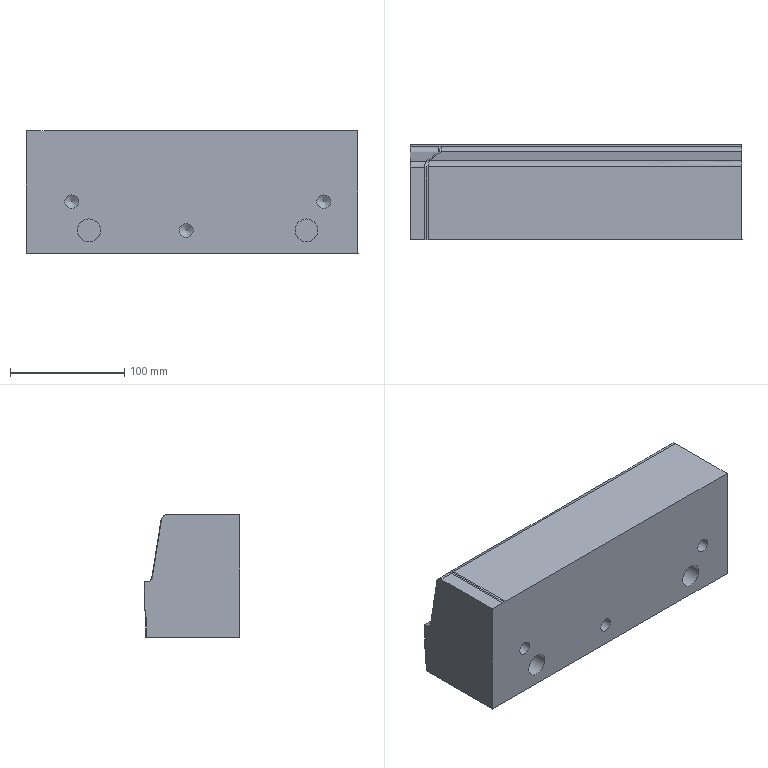Part | NX | features solid 2 | 1 solid | 33 faces | box 290 x 83.721 x 107.133 mm | volume 2375336 mm3 | plane 12 | cylinder 10 | spline 8 | cone 3 | commonest cylinder face diameters 12 x5 10 x3 20 x2
STEP:
#1=CARTESIAN_POINT('',(-215.,-160.,-50.));
#2=VERTEX_POINT('',#1);
#3=CARTESIAN_POINT('',(75.,-160.,-50.));
#4=VERTEX_POINT('',#3);
#5=CARTESIAN_POINT('',(-571.479,-160.,-50.));
#6=DIRECTION('',(1.,0.,0.));
#7=VECTOR('',#6,1000.);
#8=LINE('',#5,#7);
#9=EDGE_CURVE('',#2,#4,#8,.T.);
#10=ORIENTED_EDGE('',*,*,#9,.F.);
#11=CARTESIAN_POINT('',(-215.,-78.115,-50.));
#12=VERTEX_POINT('',#11);
#13=CARTESIAN_POINT('',(-215.,-75.471,-50.));
#14=DIRECTION('',(0.,1.,0.));
#15=VECTOR('',#14,1000.);
#16=LINE('',#13,#15);
#17=EDGE_CURVE('',#2,#12,#16,.T.);
#18=ORIENTED_EDGE('',*,*,#17,.T.);
#19=CARTESIAN_POINT('',(75.,-77.708,-50.));
#20=VERTEX_POINT('',#19);
#21=CARTESIAN_POINT('',(-215.,-78.115,-50.));
#22=CARTESIAN_POINT('',(-211.979,-78.116,-50.));
#23=CARTESIAN_POINT('',(-207.448,-78.118,-50.));
#24=CARTESIAN_POINT('',(-201.406,-78.119,-50.));
#25=CARTESIAN_POINT('',(-197.63,-78.126,-50.));
#26=CARTESIAN_POINT('',(-194.609,-78.116,-50.));
#27=CARTESIAN_POINT('',(-192.344,-78.15,-50.));
#28=CARTESIAN_POINT('',(-190.078,-78.04,-50.));
#29=CARTESIAN_POINT('',(-187.813,-77.65,-50.));
#30=CARTESIAN_POINT('',(-185.547,-77.717,-50.));
#31=CARTESIAN_POINT('',(-182.527,-77.699,-50.));
#32=CARTESIAN_POINT('',(-177.24,-77.699,-50.));
#33=CARTESIAN_POINT('',(-169.688,-77.703,-50.));
#34=CARTESIAN_POINT('',(-157.605,-77.713,-50.));
#35=CARTESIAN_POINT('',(-136.459,-77.708,-50.));
#36=CARTESIAN_POINT('',(-106.25,-77.699,-50.));
#37=CARTESIAN_POINT('',(-57.917,-77.699,-50.));
#38=CARTESIAN_POINT('',(2.5,-77.706,-50.));
#39=CARTESIAN_POINT('',(50.833,-77.708,-50.));
#40=CARTESIAN_POINT('',(75.,-77.708,-50.));
#41=B_SPLINE_CURVE_WITH_KNOTS('',3,(#21,#22,#23,#24,#25,#26,#27,#28,#29,#30,#31,#32,#33,#34,#35,#36,#37,#38,#39,#40),.UNSPECIFIED.,.F.,.F.,(4,1,1,1,1,1,1,1,1,1,1,1,1,1,1,1,1,4),(0.1494,0.1584,0.163,0.1675,0.1698,0.172,0.1743,0.1766,0.1788,0.1811,0.1856,0.1947,0.2037,0.2219,0.2581,0.2944,0.3669,0.4394),.UNSPECIFIED.);
#42=EDGE_CURVE('',#12,#20,#41,.T.);
#43=ORIENTED_EDGE('',*,*,#42,.T.);
#44=CARTESIAN_POINT('',(75.,-160.,-50.));
#45=DIRECTION('',(0.,1.,0.));
#46=VECTOR('',#45,1000.);
#47=LINE('',#44,#46);
#48=EDGE_CURVE('',#4,#20,#47,.T.);
#49=ORIENTED_EDGE('',*,*,#48,.F.);
#50=EDGE_LOOP('',(#10,#18,#43,#49));
#51=FACE_BOUND('',#50,.T.);
#52=CARTESIAN_POINT('',(-571.479,-75.471,-50.));
#53=DIRECTION('',(0.,0.,-1.));
#54=DIRECTION('',(-1.,0.,0.));
#55=AXIS2_PLACEMENT_3D('',#52,#53,#54);
#56=PLANE('',#55);
#57=ADVANCED_FACE('',(#51),#56,.T.);
#58=ORIENTED_EDGE('',*,*,#42,.F.);
#59=CARTESIAN_POINT('',(-215.,-77.915,-26.496));
#60=VERTEX_POINT('',#59);
#61=CARTESIAN_POINT('',(-215.,-78.015,-38.265));
#62=DIRECTION('',(0.,-0.008536,-1.));
#63=VECTOR('',#62,1000.);
#64=LINE('',#61,#63);
#65=EDGE_CURVE('',#12,#60,#64,.F.);
#66=ORIENTED_EDGE('',*,*,#65,.T.);
#67=CARTESIAN_POINT('',(75.,-77.507,-26.5));
#68=VERTEX_POINT('',#67);
#69=CARTESIAN_POINT('',(-215.,-77.915,-26.496));
#70=CARTESIAN_POINT('',(-211.979,-77.915,-26.496));
#71=CARTESIAN_POINT('',(-207.448,-77.918,-26.496));
#72=CARTESIAN_POINT('',(-201.406,-77.918,-26.496));
#73=CARTESIAN_POINT('',(-197.63,-77.925,-26.496));
#74=CARTESIAN_POINT('',(-194.609,-77.916,-26.496));
#75=CARTESIAN_POINT('',(-192.344,-77.949,-26.496));
#76=CARTESIAN_POINT('',(-190.078,-77.839,-26.497));
#77=CARTESIAN_POINT('',(-187.813,-77.449,-26.5));
#78=CARTESIAN_POINT('',(-185.547,-77.516,-26.499));
#79=CARTESIAN_POINT('',(-182.527,-77.499,-26.5));
#80=CARTESIAN_POINT('',(-177.24,-77.499,-26.5));
#81=CARTESIAN_POINT('',(-169.688,-77.502,-26.5));
#82=CARTESIAN_POINT('',(-157.605,-77.512,-26.5));
#83=CARTESIAN_POINT('',(-136.459,-77.507,-26.5));
#84=CARTESIAN_POINT('',(-106.25,-77.499,-26.5));
#85=CARTESIAN_POINT('',(-57.917,-77.498,-26.5));
#86=CARTESIAN_POINT('',(2.5,-77.505,-26.5));
#87=CARTESIAN_POINT('',(50.833,-77.507,-26.5));
#88=CARTESIAN_POINT('',(75.,-77.507,-26.5));
#89=B_SPLINE_CURVE_WITH_KNOTS('',3,(#69,#70,#71,#72,#73,#74,#75,#76,#77,#78,#79,#80,#81,#82,#83,#84,#85,#86,#87,#88),.UNSPECIFIED.,.F.,.F.,(4,1,1,1,1,1,1,1,1,1,1,1,1,1,1,1,1,4),(0.1353,0.1444,0.1489,0.1535,0.1557,0.158,0.1603,0.1625,0.1648,0.1671,0.1716,0.1807,0.1897,0.2078,0.2441,0.2803,0.3528,0.4253),.UNSPECIFIED.);
#90=EDGE_CURVE('',#60,#68,#89,.T.);
#91=ORIENTED_EDGE('',*,*,#90,.T.);
#92=CARTESIAN_POINT('',(75.,-77.608,-38.267));
#93=DIRECTION('',(0.,-0.008536,-1.));
#94=VECTOR('',#93,1000.);
#95=LINE('',#92,#94);
#96=EDGE_CURVE('',#20,#68,#95,.F.);
#97=ORIENTED_EDGE('',*,*,#96,.F.);
#98=EDGE_LOOP('',(#58,#66,#91,#97));
#99=FACE_BOUND('',#98,.T.);
#100=CARTESIAN_POINT('',(-215.,-77.915,-26.496));
#101=CARTESIAN_POINT('',(-215.,-78.117,-50.141));
#102=CARTESIAN_POINT('',(-211.979,-77.915,-26.496));
#103=CARTESIAN_POINT('',(-211.979,-78.117,-50.141));
#104=CARTESIAN_POINT('',(-207.449,-77.918,-26.496));
#105=CARTESIAN_POINT('',(-207.449,-78.12,-50.141));
#106=CARTESIAN_POINT('',(-201.403,-77.918,-26.496));
#107=CARTESIAN_POINT('',(-201.403,-78.12,-50.141));
#108=CARTESIAN_POINT('',(-197.637,-77.926,-26.496));
#109=CARTESIAN_POINT('',(-197.637,-78.128,-50.141));
#110=CARTESIAN_POINT('',(-194.595,-77.914,-26.496));
#111=CARTESIAN_POINT('',(-194.595,-78.116,-50.141));
#112=CARTESIAN_POINT('',(-192.394,-77.956,-26.496));
#113=CARTESIAN_POINT('',(-192.394,-78.158,-50.141));
#114=CARTESIAN_POINT('',(-189.892,-77.814,-26.497));
#115=CARTESIAN_POINT('',(-189.892,-78.016,-50.142));
#116=CARTESIAN_POINT('',(-187.778,-77.451,-26.5));
#117=CARTESIAN_POINT('',(-187.778,-77.653,-50.145));
#118=CARTESIAN_POINT('',(-185.598,-77.515,-26.499));
#119=CARTESIAN_POINT('',(-185.598,-77.717,-50.145));
#120=CARTESIAN_POINT('',(-182.526,-77.499,-26.5));
#121=CARTESIAN_POINT('',(-182.526,-77.701,-50.145));
#122=CARTESIAN_POINT('',(-177.274,-77.498,-26.5));
#123=CARTESIAN_POINT('',(-177.274,-77.7,-50.145));
#124=CARTESIAN_POINT('',(-169.704,-77.502,-26.5));
#125=CARTESIAN_POINT('',(-169.704,-77.704,-50.145));
#126=CARTESIAN_POINT('',(-157.625,-77.512,-26.5));
#127=CARTESIAN_POINT('',(-157.625,-77.714,-50.145));
#128=CARTESIAN_POINT('',(-136.473,-77.507,-26.5));
#129=CARTESIAN_POINT('',(-136.473,-77.709,-50.145));
#130=CARTESIAN_POINT('',(-106.265,-77.499,-26.5));
#131=CARTESIAN_POINT('',(-106.265,-77.701,-50.145));
#132=CARTESIAN_POINT('',(-57.927,-77.498,-26.5));
#133=CARTESIAN_POINT('',(-57.927,-77.7,-50.145));
#134=CARTESIAN_POINT('',(2.494,-77.505,-26.5));
#135=CARTESIAN_POINT('',(2.494,-77.707,-50.145));
#136=CARTESIAN_POINT('',(50.831,-77.507,-26.5));
#137=CARTESIAN_POINT('',(50.831,-77.709,-50.145));
#138=CARTESIAN_POINT('',(75.,-77.507,-26.5));
#139=CARTESIAN_POINT('',(75.,-77.709,-50.145));
#140=B_SPLINE_SURFACE_WITH_KNOTS('',3,1,((#100,#101),(#102,#103),(#104,#105),(#106,#107),(#108,#109),(#110,#111),(#112,#113),(#114,#115),(#116,#117),(#118,#119),(#120,#121),(#122,#123),(#124,#125),(#126,#127),(#128,#129),(#130,#131),(#132,#133),(#134,#135),(#136,#137),(#138,#139)),.SURF_OF_LINEAR_EXTRUSION.,.F.,.F.,.F.,(4,1,1,1,1,1,1,1,1,1,1,1,1,1,1,1,1,4),(2,2),(0.3592,0.3659,0.3692,0.3725,0.3742,0.3758,0.3775,0.3791,0.3808,0.3825,0.3858,0.3924,0.3991,0.4123,0.4389,0.4654,0.5185,0.5716),(0.,1.),.UNSPECIFIED.);
#141=ADVANCED_FACE('',(#99),#140,.T.);
#142=ORIENTED_EDGE('',*,*,#96,.T.);
#143=CARTESIAN_POINT('',(75.,-76.294,-26.51));
#144=VERTEX_POINT('',#143);
#145=CARTESIAN_POINT('',(75.,-76.914,-26.505));
#146=DIRECTION('',(0.,-1.,0.008536));
#147=VECTOR('',#146,1000.);
#148=LINE('',#145,#147);
#149=EDGE_CURVE('',#144,#68,#148,.T.);
#150=ORIENTED_EDGE('',*,*,#149,.F.);
#151=CARTESIAN_POINT('',(75.,-76.294,-1.509));
#152=VERTEX_POINT('',#151);
#153=CARTESIAN_POINT('',(75.,-76.294,-14.008));
#154=DIRECTION('',(0.,0.,-1.));
#155=VECTOR('',#154,1000.);
#156=LINE('',#153,#155);
#157=EDGE_CURVE('',#152,#144,#156,.T.);
#158=ORIENTED_EDGE('',*,*,#157,.F.);
#159=CARTESIAN_POINT('',(75.,-78.294,-1.492));
#160=VERTEX_POINT('',#159);
#161=CARTESIAN_POINT('',(75.,46.797,-2.56));
#162=DIRECTION('',(0.,1.,-0.008536));
#163=VECTOR('',#162,1000.);
#164=LINE('',#161,#163);
#165=EDGE_CURVE('',#160,#152,#164,.T.);
#166=ORIENTED_EDGE('',*,*,#165,.F.);
#167=CARTESIAN_POINT('',(75.,-83.189,2.72));
#168=VERTEX_POINT('',#167);
#169=CARTESIAN_POINT('',(75.,-78.252,3.508));
#170=DIRECTION('',(-1.,0.,0.));
#171=DIRECTION('',(0.,0.,1.));
#172=AXIS2_PLACEMENT_3D('',#169,#170,#171);
#173=CIRCLE('',#172,5.);
#174=EDGE_CURVE('',#168,#160,#173,.F.);
#175=ORIENTED_EDGE('',*,*,#174,.F.);
#176=CARTESIAN_POINT('',(75.,-91.197,52.92));
#177=VERTEX_POINT('',#176);
#178=CARTESIAN_POINT('',(75.,-87.499,29.736));
#179=DIRECTION('',(0.,0.1575,-0.9875));
#180=VECTOR('',#179,1000.);
#181=LINE('',#178,#180);
#182=EDGE_CURVE('',#177,#168,#181,.T.);
#183=ORIENTED_EDGE('',*,*,#182,.F.);
#184=CARTESIAN_POINT('',(75.,-96.134,57.133));
#185=VERTEX_POINT('',#184);
#186=CARTESIAN_POINT('',(75.,-96.134,52.133));
#187=DIRECTION('',(-1.,0.,0.));
#188=DIRECTION('',(0.,0.,1.));
#189=AXIS2_PLACEMENT_3D('',#186,#187,#188);
#190=CIRCLE('',#189,5.);
#191=EDGE_CURVE('',#177,#185,#190,.F.);
#192=ORIENTED_EDGE('',*,*,#191,.T.);
#193=CARTESIAN_POINT('',(75.,-160.,57.133));
#194=VERTEX_POINT('',#193);
#195=CARTESIAN_POINT('',(75.,-91.869,57.133));
#196=DIRECTION('',(0.,-1.,0.));
#197=VECTOR('',#196,1000.);
#198=LINE('',#195,#197);
#199=EDGE_CURVE('',#185,#194,#198,.T.);
#200=ORIENTED_EDGE('',*,*,#199,.T.);
#201=CARTESIAN_POINT('',(75.,-160.,200.));
#202=DIRECTION('',(0.,0.,1.));
#203=VECTOR('',#202,1000.);
#204=LINE('',#201,#203);
#205=EDGE_CURVE('',#4,#194,#204,.T.);
#206=ORIENTED_EDGE('',*,*,#205,.F.);
#207=ORIENTED_EDGE('',*,*,#48,.T.);
#208=EDGE_LOOP('',(#142,#150,#158,#166,#175,#183,#192,#200,#206,#207));
#209=FACE_BOUND('',#208,.T.);
#210=CARTESIAN_POINT('',(75.,360.,0.));
#211=DIRECTION('',(-1.,0.,0.));
#212=DIRECTION('',(0.,0.,1.));
#213=AXIS2_PLACEMENT_3D('',#210,#211,#212);
#214=PLANE('',#213);
#215=ADVANCED_FACE('',(#209),#214,.F.);
#216=CARTESIAN_POINT('',(-215.,-160.,57.07));
#217=VERTEX_POINT('',#216);
#218=CARTESIAN_POINT('',(-215.,-160.,200.));
#219=DIRECTION('',(0.,0.,1.));
#220=VECTOR('',#219,1000.);
#221=LINE('',#218,#220);
#222=EDGE_CURVE('',#2,#217,#221,.T.);
#223=ORIENTED_EDGE('',*,*,#222,.F.);
#224=ORIENTED_EDGE('',*,*,#9,.T.);
#225=ORIENTED_EDGE('',*,*,#205,.T.);
#226=CARTESIAN_POINT('',(-198.963,-160.,57.133));
#227=VERTEX_POINT('',#226);
#228=CARTESIAN_POINT('',(-705.,-160.,57.133));
#229=DIRECTION('',(1.,0.,0.));
#230=VECTOR('',#229,1000.);
#231=LINE('',#228,#230);
#232=EDGE_CURVE('',#227,#194,#231,.T.);
#233=ORIENTED_EDGE('',*,*,#232,.F.);
#234=CARTESIAN_POINT('',(-200.536,-160.,57.112));
#235=VERTEX_POINT('',#234);
#236=CARTESIAN_POINT('',(-703.043,-160.,50.532));
#237=DIRECTION('',(0.9999,0.,0.01309));
#238=VECTOR('',#237,1000.);
#239=LINE('',#236,#238);
#240=EDGE_CURVE('',#235,#227,#239,.T.);
#241=ORIENTED_EDGE('',*,*,#240,.F.);
#242=CARTESIAN_POINT('',(-202.104,-160.,57.07));
#243=VERTEX_POINT('',#242);
#244=CARTESIAN_POINT('',(-200.536,-160.,57.112));
#245=CARTESIAN_POINT('',(-201.059,-160.,57.095));
#246=CARTESIAN_POINT('',(-201.581,-160.,57.081));
#247=CARTESIAN_POINT('',(-202.104,-160.,57.075));
#248=B_SPLINE_CURVE_WITH_KNOTS('',3,(#244,#245,#246,#247),.UNSPECIFIED.,.F.,.F.,(4,4),(0.006154,0.007723),.UNSPECIFIED.);
#249=EDGE_CURVE('',#243,#235,#248,.F.);
#250=ORIENTED_EDGE('',*,*,#249,.F.);
#251=CARTESIAN_POINT('',(-705.,-160.,57.07));
#252=DIRECTION('',(-1.,0.,0.));
#253=VECTOR('',#252,1000.);
#254=LINE('',#251,#253);
#255=EDGE_CURVE('',#243,#217,#254,.T.);
#256=ORIENTED_EDGE('',*,*,#255,.T.);
#257=EDGE_LOOP('',(#223,#224,#225,#233,#241,#250,#256));
#258=FACE_BOUND('',#257,.T.);
#259=CARTESIAN_POINT('',(45.,-160.,1.));
#260=VERTEX_POINT('',#259);
#261=CARTESIAN_POINT('',(45.,-160.,-5.));
#262=DIRECTION('',(0.,1.,0.));
#263=DIRECTION('',(0.,0.,1.));
#264=AXIS2_PLACEMENT_3D('',#261,#262,#263);
#265=CIRCLE('',#264,6.);
#266=EDGE_CURVE('',#260,#260,#265,.T.);
#267=ORIENTED_EDGE('',*,*,#266,.T.);
#268=EDGE_LOOP('',(#267));
#269=FACE_BOUND('',#268,.T.);
#270=CARTESIAN_POINT('',(-75.,-160.,-24.));
#271=VERTEX_POINT('',#270);
#272=CARTESIAN_POINT('',(-75.,-160.,-30.));
#273=DIRECTION('',(0.,1.,0.));
#274=DIRECTION('',(0.,0.,1.));
#275=AXIS2_PLACEMENT_3D('',#272,#273,#274);
#276=CIRCLE('',#275,6.);
#277=EDGE_CURVE('',#271,#271,#276,.T.);
#278=ORIENTED_EDGE('',*,*,#277,.T.);
#279=EDGE_LOOP('',(#278));
#280=FACE_BOUND('',#279,.T.);
#281=CARTESIAN_POINT('',(-175.,-160.,1.));
#282=VERTEX_POINT('',#281);
#283=CARTESIAN_POINT('',(-175.,-160.,-5.));
#284=DIRECTION('',(0.,1.,0.));
#285=DIRECTION('',(0.,0.,1.));
#286=AXIS2_PLACEMENT_3D('',#283,#284,#285);
#287=CIRCLE('',#286,6.);
#288=EDGE_CURVE('',#282,#282,#287,.T.);
#289=ORIENTED_EDGE('',*,*,#288,.T.);
#290=EDGE_LOOP('',(#289));
#291=FACE_BOUND('',#290,.T.);
#292=CARTESIAN_POINT('',(30.,-160.,-20.));
#293=VERTEX_POINT('',#292);
#294=CARTESIAN_POINT('',(30.,-160.,-30.));
#295=DIRECTION('',(0.,1.,0.));
#296=DIRECTION('',(0.,0.,1.));
#297=AXIS2_PLACEMENT_3D('',#294,#295,#296);
#298=CIRCLE('',#297,10.);
#299=EDGE_CURVE('',#293,#293,#298,.T.);
#300=ORIENTED_EDGE('',*,*,#299,.T.);
#301=EDGE_LOOP('',(#300));
#302=FACE_BOUND('',#301,.T.);
#303=CARTESIAN_POINT('',(-160.,-160.,-20.));
#304=VERTEX_POINT('',#303);
#305=CARTESIAN_POINT('',(-160.,-160.,-30.));
#306=DIRECTION('',(0.,1.,0.));
#307=DIRECTION('',(0.,0.,1.));
#308=AXIS2_PLACEMENT_3D('',#305,#306,#307);
#309=CIRCLE('',#308,10.);
#310=EDGE_CURVE('',#304,#304,#309,.T.);
#311=ORIENTED_EDGE('',*,*,#310,.T.);
#312=EDGE_LOOP('',(#311));
#313=FACE_BOUND('',#312,.T.);
#314=CARTESIAN_POINT('',(-705.,-160.,200.));
#315=DIRECTION('',(0.,1.,0.));
#316=DIRECTION('',(0.,0.,1.));
#317=AXIS2_PLACEMENT_3D('',#314,#315,#316);
#318=PLANE('',#317);
#319=ADVANCED_FACE('',(#258,#269,#280,#291,#302,#313),#318,.F.);
#320=CARTESIAN_POINT('',(-215.,-76.704,-26.506));
#321=VERTEX_POINT('',#320);
#322=CARTESIAN_POINT('',(-215.,-76.914,-26.505));
#323=DIRECTION('',(0.,-1.,0.008536));
#324=VECTOR('',#323,1000.);
#325=LINE('',#322,#324);
#326=EDGE_CURVE('',#321,#60,#325,.T.);
#327=ORIENTED_EDGE('',*,*,#326,.T.);
#328=ORIENTED_EDGE('',*,*,#65,.F.);
#329=ORIENTED_EDGE('',*,*,#17,.F.);
#330=ORIENTED_EDGE('',*,*,#222,.T.);
#331=CARTESIAN_POINT('',(-215.,-96.529,57.07));
#332=VERTEX_POINT('',#331);
#333=CARTESIAN_POINT('',(-215.,-392.264,57.07));
#334=DIRECTION('',(0.,1.,0.));
#335=VECTOR('',#334,1000.);
#336=LINE('',#333,#335);
#337=EDGE_CURVE('',#217,#332,#336,.T.);
#338=ORIENTED_EDGE('',*,*,#337,.T.);
#339=CARTESIAN_POINT('',(-215.,-91.592,52.857));
#340=VERTEX_POINT('',#339);
#341=CARTESIAN_POINT('',(-215.,-96.529,52.07));
#342=DIRECTION('',(-1.,0.,0.));
#343=DIRECTION('',(0.,0.,1.));
#344=AXIS2_PLACEMENT_3D('',#341,#342,#343);
#345=CIRCLE('',#344,5.);
#346=EDGE_CURVE('',#340,#332,#345,.F.);
#347=ORIENTED_EDGE('',*,*,#346,.F.);
#348=CARTESIAN_POINT('',(-215.,-83.595,2.724));
#349=VERTEX_POINT('',#348);
#350=CARTESIAN_POINT('',(-215.,-79.399,-23.581));
#351=DIRECTION('',(0.,0.1575,-0.9875));
#352=VECTOR('',#351,1000.);
#353=LINE('',#350,#352);
#354=EDGE_CURVE('',#340,#349,#353,.T.);
#355=ORIENTED_EDGE('',*,*,#354,.T.);
#356=CARTESIAN_POINT('',(-215.,-78.7,-1.488));
#357=VERTEX_POINT('',#356);
#358=CARTESIAN_POINT('',(-215.,-78.657,3.511));
#359=DIRECTION('',(-1.,0.,0.));
#360=DIRECTION('',(0.,0.,1.));
#361=AXIS2_PLACEMENT_3D('',#358,#359,#360);
#362=CIRCLE('',#361,5.);
#363=EDGE_CURVE('',#349,#357,#362,.F.);
#364=ORIENTED_EDGE('',*,*,#363,.T.);
#365=CARTESIAN_POINT('',(-215.,-76.704,-1.506));
#366=VERTEX_POINT('',#365);
#367=CARTESIAN_POINT('',(-215.,46.797,-2.56));
#368=DIRECTION('',(0.,1.,-0.008536));
#369=VECTOR('',#368,1000.);
#370=LINE('',#367,#369);
#371=EDGE_CURVE('',#357,#366,#370,.T.);
#372=ORIENTED_EDGE('',*,*,#371,.T.);
#373=CARTESIAN_POINT('',(-215.,-76.704,-14.008));
#374=DIRECTION('',(0.,0.,-1.));
#375=VECTOR('',#374,1000.);
#376=LINE('',#373,#375);
#377=EDGE_CURVE('',#366,#321,#376,.T.);
#378=ORIENTED_EDGE('',*,*,#377,.T.);
#379=EDGE_LOOP('',(#327,#328,#329,#330,#338,#347,#355,#364,#372,#378));
#380=FACE_BOUND('',#379,.T.);
#381=CARTESIAN_POINT('',(-215.,360.,0.));
#382=DIRECTION('',(-1.,0.,0.));
#383=DIRECTION('',(0.,0.,1.));
#384=AXIS2_PLACEMENT_3D('',#381,#382,#383);
#385=PLANE('',#384);
#386=ADVANCED_FACE('',(#380),#385,.T.);
#387=CARTESIAN_POINT('',(-199.628,-91.395,52.891));
#388=VERTEX_POINT('',#387);
#389=CARTESIAN_POINT('',(-198.056,-91.197,52.92));
#390=VERTEX_POINT('',#389);
#391=CARTESIAN_POINT('',(-199.628,-91.395,52.894));
#392=CARTESIAN_POINT('',(-199.206,-91.287,52.907));
#393=CARTESIAN_POINT('',(-198.679,-91.197,52.92));
#394=CARTESIAN_POINT('',(-198.056,-91.197,52.92));
#395=B_SPLINE_CURVE_WITH_KNOTS('',3,(#391,#392,#393,#394),.UNSPECIFIED.,.F.,.F.,(4,4),(0.6644,1.),.UNSPECIFIED.);
#396=EDGE_CURVE('',#388,#390,#395,.T.);
#397=ORIENTED_EDGE('',*,*,#396,.T.);
#398=CARTESIAN_POINT('',(-196.309,-89.902,44.803));
#399=VERTEX_POINT('',#398);
#400=CARTESIAN_POINT('',(-196.309,-89.902,44.803));
#401=CARTESIAN_POINT('',(-196.892,-90.333,47.509));
#402=CARTESIAN_POINT('',(-197.474,-90.765,50.215));
#403=CARTESIAN_POINT('',(-198.056,-91.197,52.92));
#404=B_SPLINE_CURVE_WITH_KNOTS('',3,(#400,#401,#402,#403),.UNSPECIFIED.,.F.,.F.,(4,4),(0.,1.),.UNSPECIFIED.);
#405=EDGE_CURVE('',#399,#390,#404,.T.);
#406=ORIENTED_EDGE('',*,*,#405,.F.);
#407=CARTESIAN_POINT('',(-194.188,-88.33,34.95));
#408=VERTEX_POINT('',#407);
#409=CARTESIAN_POINT('',(-194.188,-88.33,34.95));
#410=CARTESIAN_POINT('',(-194.895,-88.854,38.234));
#411=CARTESIAN_POINT('',(-195.602,-89.378,41.518));
#412=CARTESIAN_POINT('',(-196.309,-89.902,44.803));
#413=B_SPLINE_CURVE_WITH_KNOTS('',3,(#409,#410,#411,#412),.UNSPECIFIED.,.F.,.F.,(4,4),(0.,1.),.UNSPECIFIED.);
#414=EDGE_CURVE('',#408,#399,#413,.T.);
#415=ORIENTED_EDGE('',*,*,#414,.F.);
#416=CARTESIAN_POINT('',(-187.251,-83.189,2.72));
#417=VERTEX_POINT('',#416);
#418=CARTESIAN_POINT('',(-187.251,-83.189,2.72));
#419=CARTESIAN_POINT('',(-189.564,-84.903,13.463));
#420=CARTESIAN_POINT('',(-191.876,-86.617,24.207));
#421=CARTESIAN_POINT('',(-194.188,-88.33,34.95));
#422=B_SPLINE_CURVE_WITH_KNOTS('',3,(#418,#419,#420,#421),.UNSPECIFIED.,.F.,.F.,(4,4),(0.,1.),.UNSPECIFIED.);
#423=EDGE_CURVE('',#417,#408,#422,.T.);
#424=ORIENTED_EDGE('',*,*,#423,.F.);
#425=CARTESIAN_POINT('',(-188.891,-83.438,3.013));
#426=VERTEX_POINT('',#425);
#427=CARTESIAN_POINT('',(-188.891,-83.438,3.013));
#428=CARTESIAN_POINT('',(-188.315,-83.277,2.9));
#429=CARTESIAN_POINT('',(-187.761,-83.202,2.803));
#430=CARTESIAN_POINT('',(-187.251,-83.189,2.72));
#431=B_SPLINE_CURVE_WITH_KNOTS('',3,(#427,#428,#429,#430),.UNSPECIFIED.,.F.,.F.,(4,4),(0.,1.),.UNSPECIFIED.);
#432=EDGE_CURVE('',#417,#426,#431,.F.);
#433=ORIENTED_EDGE('',*,*,#432,.T.);
#434=CARTESIAN_POINT('',(-195.756,-88.526,34.905));
#435=VERTEX_POINT('',#434);
#436=CARTESIAN_POINT('',(-195.756,-88.526,34.905));
#437=CARTESIAN_POINT('',(-193.468,-86.83,24.274));
#438=CARTESIAN_POINT('',(-191.18,-85.134,13.643));
#439=CARTESIAN_POINT('',(-188.891,-83.438,3.013));
#440=B_SPLINE_CURVE_WITH_KNOTS('',3,(#436,#437,#438,#439),.UNSPECIFIED.,.F.,.F.,(4,4),(0.,1.),.UNSPECIFIED.);
#441=EDGE_CURVE('',#426,#435,#440,.F.);
#442=ORIENTED_EDGE('',*,*,#441,.T.);
#443=CARTESIAN_POINT('',(-197.877,-90.097,44.758));
#444=VERTEX_POINT('',#443);
#445=CARTESIAN_POINT('',(-190.129,-84.356,8.763));
#446=DIRECTION('',(-0.2079,-0.1541,0.9659));
#447=VECTOR('',#446,1000.);
#448=LINE('',#445,#447);
#449=EDGE_CURVE('',#435,#444,#448,.T.);
#450=ORIENTED_EDGE('',*,*,#449,.T.);
#451=CARTESIAN_POINT('',(-199.628,-91.395,52.894));
#452=CARTESIAN_POINT('',(-199.044,-90.962,50.182));
#453=CARTESIAN_POINT('',(-198.461,-90.53,47.47));
#454=CARTESIAN_POINT('',(-197.877,-90.097,44.758));
#455=B_SPLINE_CURVE_WITH_KNOTS('',3,(#451,#452,#453,#454),.UNSPECIFIED.,.F.,.F.,(4,4),(0.,1.),.UNSPECIFIED.);
#456=EDGE_CURVE('',#444,#388,#455,.F.);
#457=ORIENTED_EDGE('',*,*,#456,.T.);
#458=EDGE_LOOP('',(#397,#406,#415,#424,#433,#442,#450,#457));
#459=FACE_BOUND('',#458,.T.);
#460=CARTESIAN_POINT('',(-188.626,-90.134,8.164));
#461=DIRECTION('',(-0.2079,-0.1541,0.9659));
#462=DIRECTION('',(0.9781,-0.03275,0.2053));
#463=AXIS2_PLACEMENT_3D('',#460,#461,#462);
#464=CYLINDRICAL_SURFACE('',#463,6.);
#465=ADVANCED_FACE('',(#459),#464,.T.);
#466=ORIENTED_EDGE('',*,*,#191,.F.);
#467=CARTESIAN_POINT('',(-198.056,-91.197,52.92));
#468=CARTESIAN_POINT('',(-107.038,-91.197,52.92));
#469=CARTESIAN_POINT('',(-16.019,-91.197,52.92));
#470=CARTESIAN_POINT('',(75.,-91.197,52.92));
#471=B_SPLINE_CURVE_WITH_KNOTS('',3,(#467,#468,#469,#470),.UNSPECIFIED.,.F.,.F.,(4,4),(0.,0.2731),.UNSPECIFIED.);
#472=EDGE_CURVE('',#390,#177,#471,.T.);
#473=ORIENTED_EDGE('',*,*,#472,.F.);
#474=CARTESIAN_POINT('',(-198.963,-96.134,57.132));
#475=VERTEX_POINT('',#474);
#476=CARTESIAN_POINT('',(-198.963,-96.133,57.132));
#477=CARTESIAN_POINT('',(-198.958,-94.944,57.111));
#478=CARTESIAN_POINT('',(-198.774,-92.575,56.253));
#479=CARTESIAN_POINT('',(-198.303,-91.389,54.067));
#480=CARTESIAN_POINT('',(-198.056,-91.197,52.92));
#481=B_SPLINE_CURVE_WITH_KNOTS('',3,(#476,#477,#478,#479,#480),.UNSPECIFIED.,.F.,.F.,(4,1,4),(0.,0.5,1.),.UNSPECIFIED.);
#482=EDGE_CURVE('',#475,#390,#481,.T.);
#483=ORIENTED_EDGE('',*,*,#482,.F.);
#484=CARTESIAN_POINT('',(75.,-96.134,57.133));
#485=CARTESIAN_POINT('',(-16.321,-96.134,57.133));
#486=CARTESIAN_POINT('',(-107.642,-96.134,57.133));
#487=CARTESIAN_POINT('',(-198.963,-96.134,57.133));
#488=B_SPLINE_CURVE_WITH_KNOTS('',3,(#484,#485,#486,#487),.UNSPECIFIED.,.F.,.F.,(4,4),(0.6686,0.9426),.UNSPECIFIED.);
#489=EDGE_CURVE('',#185,#475,#488,.T.);
#490=ORIENTED_EDGE('',*,*,#489,.F.);
#491=EDGE_LOOP('',(#466,#473,#483,#490));
#492=FACE_BOUND('',#491,.T.);
#493=CARTESIAN_POINT('',(75.,-91.197,52.92));
#494=CARTESIAN_POINT('',(75.,-91.869,57.133));
#495=CARTESIAN_POINT('',(75.,-96.134,57.133));
#496=CARTESIAN_POINT('',(-16.869,-91.197,52.92));
#497=CARTESIAN_POINT('',(-16.869,-91.869,57.133));
#498=CARTESIAN_POINT('',(-16.869,-96.134,57.133));
#499=CARTESIAN_POINT('',(-108.738,-91.197,52.92));
#500=CARTESIAN_POINT('',(-108.738,-91.869,57.133));
#501=CARTESIAN_POINT('',(-108.738,-96.134,57.133));
#502=CARTESIAN_POINT('',(-200.607,-91.197,52.92));
#503=CARTESIAN_POINT('',(-200.607,-91.869,57.133));
#504=CARTESIAN_POINT('',(-200.607,-96.134,57.133));
#505=(BOUNDED_SURFACE()B_SPLINE_SURFACE(3,2,((#493,#494,#495),(#496,#497,#498),(#499,#500,#501),(#502,#503,#504)),.UNSPECIFIED.,.F.,.F.,.F.)B_SPLINE_SURFACE_WITH_KNOTS((4,4),(3,3),(0.7843,1.06),(0.,1.),.PIECEWISE_BEZIER_KNOTS.)GEOMETRIC_REPRESENTATION_ITEM()RATIONAL_B_SPLINE_SURFACE(((1.,0.7608,1.),(1.,0.7608,1.),(1.,0.7608,1.),(1.,0.7608,1.)))REPRESENTATION_ITEM('')SURFACE());
#506=ADVANCED_FACE('',(#492),#505,.T.);
#507=ORIENTED_EDGE('',*,*,#472,.T.);
#508=ORIENTED_EDGE('',*,*,#182,.T.);
#509=CARTESIAN_POINT('',(-187.251,-83.189,2.72));
#510=CARTESIAN_POINT('',(-99.834,-83.189,2.72));
#511=CARTESIAN_POINT('',(-12.417,-83.189,2.72));
#512=CARTESIAN_POINT('',(75.,-83.189,2.72));
#513=B_SPLINE_CURVE_WITH_KNOTS('',3,(#509,#510,#511,#512),.UNSPECIFIED.,.F.,.F.,(4,4),(0.,0.3113),.UNSPECIFIED.);
#514=EDGE_CURVE('',#417,#168,#513,.T.);
#515=ORIENTED_EDGE('',*,*,#514,.F.);
#516=ORIENTED_EDGE('',*,*,#423,.T.);
#517=ORIENTED_EDGE('',*,*,#414,.T.);
#518=ORIENTED_EDGE('',*,*,#405,.T.);
#519=EDGE_LOOP('',(#507,#508,#515,#516,#517,#518));
#520=FACE_BOUND('',#519,.T.);
#521=CARTESIAN_POINT('',(808.196,-82.695,-0.3814));
#522=CARTESIAN_POINT('',(-199.284,-82.695,-0.3814));
#523=CARTESIAN_POINT('',(808.196,-92.303,59.853));
#524=CARTESIAN_POINT('',(-199.284,-92.303,59.853));
#525=B_SPLINE_SURFACE_WITH_KNOTS('',1,1,((#521,#522),(#523,#524)),.PLANE_SURF.,.F.,.F.,.F.,(2,2),(2,2),(-0.06964,1.283),(-0.1722,1.),.UNSPECIFIED.);
#526=ADVANCED_FACE('',(#520),#525,.F.);
#527=CARTESIAN_POINT('',(-202.105,-96.529,57.073));
#528=VERTEX_POINT('',#527);
#529=CARTESIAN_POINT('',(-200.536,-96.332,57.107));
#530=VERTEX_POINT('',#529);
#531=CARTESIAN_POINT('',(-202.104,-96.529,57.075));
#532=CARTESIAN_POINT('',(-201.578,-96.529,57.081));
#533=CARTESIAN_POINT('',(-201.072,-96.436,57.094));
#534=CARTESIAN_POINT('',(-200.536,-96.332,57.112));
#535=B_SPLINE_CURVE_WITH_KNOTS('',3,(#531,#532,#533,#534),.UNSPECIFIED.,.F.,.F.,(4,4),(0.,0.9789),.UNSPECIFIED.);
#536=EDGE_CURVE('',#528,#530,#535,.T.);
#537=ORIENTED_EDGE('',*,*,#536,.T.);
#538=CARTESIAN_POINT('',(-200.536,-96.332,57.112));
#539=CARTESIAN_POINT('',(-200.011,-96.266,57.119));
#540=CARTESIAN_POINT('',(-199.487,-96.199,57.126));
#541=CARTESIAN_POINT('',(-198.963,-96.133,57.133));
#542=B_SPLINE_CURVE_WITH_KNOTS('',3,(#538,#539,#540,#541),.UNSPECIFIED.,.F.,.F.,(4,4),(0.,1.),.UNSPECIFIED.);
#543=EDGE_CURVE('',#530,#475,#542,.T.);
#544=ORIENTED_EDGE('',*,*,#543,.T.);
#545=ORIENTED_EDGE('',*,*,#482,.T.);
#546=ORIENTED_EDGE('',*,*,#396,.F.);
#547=CARTESIAN_POINT('',(-201.198,-91.592,52.857));
#548=VERTEX_POINT('',#547);
#549=CARTESIAN_POINT('',(-201.198,-91.592,52.857));
#550=CARTESIAN_POINT('',(-200.668,-91.592,52.859));
#551=CARTESIAN_POINT('',(-200.139,-91.525,52.87));
#552=CARTESIAN_POINT('',(-199.627,-91.394,52.889));
#553=B_SPLINE_CURVE_WITH_KNOTS('',3,(#549,#550,#551,#552),.UNSPECIFIED.,.F.,.F.,(4,4),(0.,0.9602),.UNSPECIFIED.);
#554=EDGE_CURVE('',#548,#388,#553,.T.);
#555=ORIENTED_EDGE('',*,*,#554,.F.);
#556=CARTESIAN_POINT('',(-201.198,-91.592,52.857));
#557=CARTESIAN_POINT('',(-201.5,-91.816,54.262));
#558=CARTESIAN_POINT('',(-201.953,-93.438,56.537));
#559=CARTESIAN_POINT('',(-202.104,-95.597,57.07));
#560=CARTESIAN_POINT('',(-202.104,-96.529,57.07));
#561=B_SPLINE_CURVE_WITH_KNOTS('',3,(#556,#557,#558,#559,#560),.UNSPECIFIED.,.F.,.F.,(4,1,4),(0.,0.5,1.),.UNSPECIFIED.);
#562=EDGE_CURVE('',#528,#548,#561,.F.);
#563=ORIENTED_EDGE('',*,*,#562,.F.);
#564=EDGE_LOOP('',(#537,#544,#545,#546,#555,#563));
#565=FACE_BOUND('',#564,.T.);
#566=CARTESIAN_POINT('',(-202.104,-96.53,57.07));
#567=CARTESIAN_POINT('',(-202.104,-96.232,57.068));
#568=CARTESIAN_POINT('',(-202.092,-95.638,57.013));
#569=CARTESIAN_POINT('',(-202.042,-94.775,56.781));
#570=CARTESIAN_POINT('',(-201.959,-93.97,56.396));
#571=CARTESIAN_POINT('',(-201.81,-93.008,55.705));
#572=CARTESIAN_POINT('',(-201.561,-92.078,54.547));
#573=CARTESIAN_POINT('',(-201.321,-91.687,53.431));
#574=CARTESIAN_POINT('',(-201.198,-91.591,52.857));
#575=CARTESIAN_POINT('',(-201.576,-96.524,57.071));
#576=CARTESIAN_POINT('',(-201.575,-96.227,57.068));
#577=CARTESIAN_POINT('',(-201.564,-95.632,57.016));
#578=CARTESIAN_POINT('',(-201.513,-94.77,56.781));
#579=CARTESIAN_POINT('',(-201.431,-93.965,56.397));
#580=CARTESIAN_POINT('',(-201.282,-93.002,55.706));
#581=CARTESIAN_POINT('',(-201.033,-92.073,54.548));
#582=CARTESIAN_POINT('',(-200.792,-91.682,53.432));
#583=CARTESIAN_POINT('',(-200.669,-91.586,52.858));
#584=CARTESIAN_POINT('',(-200.534,-96.332,57.101));
#585=CARTESIAN_POINT('',(-200.533,-96.034,57.097));
#586=CARTESIAN_POINT('',(-200.523,-95.439,57.05));
#587=CARTESIAN_POINT('',(-200.471,-94.577,56.81));
#588=CARTESIAN_POINT('',(-200.388,-93.772,56.427));
#589=CARTESIAN_POINT('',(-200.24,-92.808,55.737));
#590=CARTESIAN_POINT('',(-199.991,-91.879,54.579));
#591=CARTESIAN_POINT('',(-199.751,-91.487,53.463));
#592=CARTESIAN_POINT('',(-199.627,-91.391,52.889));
#593=CARTESIAN_POINT('',(-199.491,-96.139,57.131));
#594=CARTESIAN_POINT('',(-199.49,-95.842,57.126));
#595=CARTESIAN_POINT('',(-199.481,-95.247,57.084));
#596=CARTESIAN_POINT('',(-199.429,-94.387,56.839));
#597=CARTESIAN_POINT('',(-199.346,-93.583,56.456));
#598=CARTESIAN_POINT('',(-199.198,-92.619,55.768));
#599=CARTESIAN_POINT('',(-198.949,-91.693,54.609));
#600=CARTESIAN_POINT('',(-198.708,-91.303,53.492));
#601=CARTESIAN_POINT('',(-198.585,-91.207,52.919));
#602=CARTESIAN_POINT('',(-198.963,-96.133,57.132));
#603=CARTESIAN_POINT('',(-198.962,-95.836,57.127));
#604=CARTESIAN_POINT('',(-198.953,-95.241,57.086));
#605=CARTESIAN_POINT('',(-198.9,-94.38,56.84));
#606=CARTESIAN_POINT('',(-198.817,-93.576,56.457));
#607=CARTESIAN_POINT('',(-198.669,-92.611,55.769));
#608=CARTESIAN_POINT('',(-198.42,-91.684,54.61));
#609=CARTESIAN_POINT('',(-198.18,-91.293,53.494));
#610=CARTESIAN_POINT('',(-198.056,-91.197,52.92));
#611=B_SPLINE_SURFACE_WITH_KNOTS('',3,3,((#566,#567,#568,#569,#570,#571,#572,#573,#574),(#575,#576,#577,#578,#579,#580,#581,#582,#583),(#584,#585,#586,#587,#588,#589,#590,#591,#592),(#593,#594,#595,#596,#597,#598,#599,#600,#601),(#602,#603,#604,#605,#606,#607,#608,#609,#610)),.UNSPECIFIED.,.F.,.F.,.F.,(4,1,4),(4,1,1,1,1,1,4),(0.,0.5,1.),(0.,0.125,0.25,0.375,0.5,0.75,1.),.UNSPECIFIED.);
#612=ADVANCED_FACE('',(#565),#611,.T.);
#613=CARTESIAN_POINT('',(-199.445,-90.293,44.717));
#614=VERTEX_POINT('',#613);
#615=CARTESIAN_POINT('',(-199.445,-90.293,44.717));
#616=CARTESIAN_POINT('',(-200.029,-90.726,47.431));
#617=CARTESIAN_POINT('',(-200.613,-91.159,50.144));
#618=CARTESIAN_POINT('',(-201.198,-91.592,52.857));
#619=B_SPLINE_CURVE_WITH_KNOTS('',3,(#615,#616,#617,#618),.UNSPECIFIED.,.F.,.F.,(4,4),(0.,1.),.UNSPECIFIED.);
#620=EDGE_CURVE('',#614,#548,#619,.T.);
#621=ORIENTED_EDGE('',*,*,#620,.T.);
#622=ORIENTED_EDGE('',*,*,#554,.T.);
#623=ORIENTED_EDGE('',*,*,#456,.F.);
#624=ORIENTED_EDGE('',*,*,#449,.F.);
#625=ORIENTED_EDGE('',*,*,#441,.F.);
#626=CARTESIAN_POINT('',(-190.407,-83.595,2.724));
#627=VERTEX_POINT('',#626);
#628=CARTESIAN_POINT('',(-188.891,-83.438,3.013));
#629=CARTESIAN_POINT('',(-189.385,-83.556,2.908));
#630=CARTESIAN_POINT('',(-189.896,-83.609,2.811));
#631=CARTESIAN_POINT('',(-190.407,-83.595,2.724));
#632=B_SPLINE_CURVE_WITH_KNOTS('',3,(#628,#629,#630,#631),.UNSPECIFIED.,.F.,.F.,(4,4),(0.000000012,1.),.UNSPECIFIED.);
#633=EDGE_CURVE('',#627,#426,#632,.F.);
#634=ORIENTED_EDGE('',*,*,#633,.F.);
#635=CARTESIAN_POINT('',(-197.324,-88.721,34.86));
#636=VERTEX_POINT('',#635);
#637=CARTESIAN_POINT('',(-190.407,-83.595,2.724));
#638=CARTESIAN_POINT('',(-192.712,-85.304,13.436));
#639=CARTESIAN_POINT('',(-195.018,-87.012,24.148));
#640=CARTESIAN_POINT('',(-197.324,-88.721,34.86));
#641=B_SPLINE_CURVE_WITH_KNOTS('',3,(#637,#638,#639,#640),.UNSPECIFIED.,.F.,.F.,(4,4),(0.,1.),.UNSPECIFIED.);
#642=EDGE_CURVE('',#627,#636,#641,.T.);
#643=ORIENTED_EDGE('',*,*,#642,.T.);
#644=CARTESIAN_POINT('',(-189.955,-83.26,0.6241));
#645=CARTESIAN_POINT('',(-190.407,-83.595,2.724));
#646=CARTESIAN_POINT('',(-197.324,-88.721,34.86));
#647=CARTESIAN_POINT('',(-199.897,-90.628,46.817));
#648=B_SPLINE_CURVE_WITH_KNOTS('',1,(#644,#645,#646,#647),.UNSPECIFIED.,.F.,.F.,(2,1,1,2),(-0.06534,0.,1.,1.372),.PIECEWISE_BEZIER_KNOTS.);
#649=EDGE_CURVE('',#636,#614,#648,.T.);
#650=ORIENTED_EDGE('',*,*,#649,.T.);
#651=EDGE_LOOP('',(#621,#622,#623,#624,#625,#634,#643,#650));
#652=FACE_BOUND('',#651,.T.);
#653=CARTESIAN_POINT('',(-195.963,-81.787,29.482));
#654=DIRECTION('',(0.2079,0.1541,-0.9659));
#655=DIRECTION('',(-0.9781,0.03275,-0.2053));
#656=AXIS2_PLACEMENT_3D('',#653,#654,#655);
#657=CYLINDRICAL_SURFACE('',#656,6.);
#658=ADVANCED_FACE('',(#652),#657,.F.);
#659=ORIENTED_EDGE('',*,*,#514,.T.);
#660=ORIENTED_EDGE('',*,*,#174,.T.);
#661=CARTESIAN_POINT('',(-187.251,-78.294,-1.492));
#662=VERTEX_POINT('',#661);
#663=CARTESIAN_POINT('',(75.,-78.294,-1.492));
#664=CARTESIAN_POINT('',(-12.417,-78.294,-1.492));
#665=CARTESIAN_POINT('',(-99.834,-78.294,-1.492));
#666=CARTESIAN_POINT('',(-187.251,-78.294,-1.492));
#667=B_SPLINE_CURVE_WITH_KNOTS('',3,(#663,#664,#665,#666),.UNSPECIFIED.,.F.,.F.,(4,4),(0.6888,1.),.UNSPECIFIED.);
#668=EDGE_CURVE('',#160,#662,#667,.T.);
#669=ORIENTED_EDGE('',*,*,#668,.T.);
#670=CARTESIAN_POINT('',(-187.251,-78.294,-1.492));
#671=CARTESIAN_POINT('',(-187.251,-79.464,-1.482));
#672=CARTESIAN_POINT('',(-187.251,-81.791,-0.6055));
#673=CARTESIAN_POINT('',(-187.251,-83.005,1.565));
#674=CARTESIAN_POINT('',(-187.251,-83.189,2.72));
#675=B_SPLINE_CURVE_WITH_KNOTS('',3,(#670,#671,#672,#673,#674),.UNSPECIFIED.,.F.,.F.,(4,1,4),(0.,0.5,1.),.UNSPECIFIED.);
#676=EDGE_CURVE('',#662,#417,#675,.T.);
#677=ORIENTED_EDGE('',*,*,#676,.T.);
#678=EDGE_LOOP('',(#659,#660,#669,#677));
#679=FACE_BOUND('',#678,.T.);
#680=CARTESIAN_POINT('',(6000655.556,-78.252,3.508));
#681=DIRECTION('',(-1.,0.,0.));
#682=DIRECTION('',(0.,-0.1575,0.9875));
#683=AXIS2_PLACEMENT_3D('',#680,#681,#682);
#684=CYLINDRICAL_SURFACE('',#683,5.);
#685=ADVANCED_FACE('',(#679),#684,.F.);
#686=ORIENTED_EDGE('',*,*,#676,.F.);
#687=CARTESIAN_POINT('',(-190.144,-78.666,-1.489));
#688=VERTEX_POINT('',#687);
#689=CARTESIAN_POINT('',(-187.251,-78.294,-1.492));
#690=CARTESIAN_POINT('',(-188.227,-78.294,-1.492));
#691=CARTESIAN_POINT('',(-189.191,-78.418,-1.491));
#692=CARTESIAN_POINT('',(-190.144,-78.666,-1.489));
#693=B_SPLINE_CURVE_WITH_KNOTS('',3,(#689,#690,#691,#692),.UNSPECIFIED.,.F.,.F.,(4,4),(0.,1.),.UNSPECIFIED.);
#694=EDGE_CURVE('',#662,#688,#693,.T.);
#695=ORIENTED_EDGE('',*,*,#694,.T.);
#696=CARTESIAN_POINT('',(-188.891,-83.438,3.013));
#697=CARTESIAN_POINT('',(-188.925,-83.322,1.8));
#698=CARTESIAN_POINT('',(-189.224,-82.19,-0.5258));
#699=CARTESIAN_POINT('',(-189.837,-79.846,-1.479));
#700=CARTESIAN_POINT('',(-190.144,-78.666,-1.489));
#701=B_SPLINE_CURVE_WITH_KNOTS('',3,(#696,#697,#698,#699,#700),.UNSPECIFIED.,.F.,.F.,(4,1,4),(0.,0.5,1.),.UNSPECIFIED.);
#702=EDGE_CURVE('',#426,#688,#701,.T.);
#703=ORIENTED_EDGE('',*,*,#702,.F.);
#704=ORIENTED_EDGE('',*,*,#432,.F.);
#705=EDGE_LOOP('',(#686,#695,#703,#704));
#706=FACE_BOUND('',#705,.T.);
#707=CARTESIAN_POINT('',(-190.144,-78.666,-1.489));
#708=CARTESIAN_POINT('',(-189.959,-79.374,-1.483));
#709=CARTESIAN_POINT('',(-189.775,-80.081,-1.343));
#710=CARTESIAN_POINT('',(-189.599,-80.754,-1.07));
#711=CARTESIAN_POINT('',(-189.28,-81.974,-0.2814));
#712=CARTESIAN_POINT('',(-189.051,-82.845,0.902));
#713=CARTESIAN_POINT('',(-188.965,-83.169,1.571));
#714=CARTESIAN_POINT('',(-188.911,-83.368,2.285));
#715=CARTESIAN_POINT('',(-188.891,-83.438,3.013));
#716=CARTESIAN_POINT('',(-189.579,-78.519,-1.49));
#717=CARTESIAN_POINT('',(-189.432,-79.23,-1.484));
#718=CARTESIAN_POINT('',(-189.285,-79.94,-1.346));
#719=CARTESIAN_POINT('',(-189.144,-80.618,-1.078));
#720=CARTESIAN_POINT('',(-188.888,-81.846,-0.3022));
#721=CARTESIAN_POINT('',(-188.703,-82.729,0.8639));
#722=CARTESIAN_POINT('',(-188.633,-83.062,1.523));
#723=CARTESIAN_POINT('',(-188.588,-83.269,2.229));
#724=CARTESIAN_POINT('',(-188.57,-83.348,2.95));
#725=CARTESIAN_POINT('',(-189.004,-78.408,-1.491));
#726=CARTESIAN_POINT('',(-188.894,-79.119,-1.485));
#727=CARTESIAN_POINT('',(-188.784,-79.83,-1.35));
#728=CARTESIAN_POINT('',(-188.679,-80.509,-1.085));
#729=CARTESIAN_POINT('',(-188.487,-81.743,-0.322));
#730=CARTESIAN_POINT('',(-188.347,-82.636,0.8272));
#731=CARTESIAN_POINT('',(-188.293,-82.975,1.478));
#732=CARTESIAN_POINT('',(-188.259,-83.19,2.175));
#733=CARTESIAN_POINT('',(-188.244,-83.278,2.889));
#734=CARTESIAN_POINT('',(-188.423,-78.332,-1.492));
#735=CARTESIAN_POINT('',(-188.35,-79.043,-1.486));
#736=CARTESIAN_POINT('',(-188.277,-79.753,-1.352));
#737=CARTESIAN_POINT('',(-188.207,-80.431,-1.092));
#738=CARTESIAN_POINT('',(-188.079,-81.666,-0.3409));
#739=CARTESIAN_POINT('',(-187.985,-82.566,0.7921));
#740=CARTESIAN_POINT('',(-187.949,-82.909,1.434));
#741=CARTESIAN_POINT('',(-187.925,-83.131,2.124));
#742=CARTESIAN_POINT('',(-187.914,-83.227,2.83));
#743=CARTESIAN_POINT('',(-187.837,-78.294,-1.492));
#744=CARTESIAN_POINT('',(-187.801,-79.002,-1.486));
#745=CARTESIAN_POINT('',(-187.765,-79.708,-1.355));
#746=CARTESIAN_POINT('',(-187.73,-80.384,-1.099));
#747=CARTESIAN_POINT('',(-187.666,-81.616,-0.3588));
#748=CARTESIAN_POINT('',(-187.619,-82.519,0.7587));
#749=CARTESIAN_POINT('',(-187.601,-82.866,1.393));
#750=CARTESIAN_POINT('',(-187.588,-83.094,2.074));
#751=CARTESIAN_POINT('',(-187.582,-83.198,2.774));
#752=CARTESIAN_POINT('',(-187.251,-78.294,-1.492));
#753=CARTESIAN_POINT('',(-187.251,-78.996,-1.486));
#754=CARTESIAN_POINT('',(-187.251,-79.697,-1.357));
#755=CARTESIAN_POINT('',(-187.251,-80.368,-1.105));
#756=CARTESIAN_POINT('',(-187.251,-81.593,-0.3754));
#757=CARTESIAN_POINT('',(-187.251,-82.497,0.7272));
#758=CARTESIAN_POINT('',(-187.251,-82.847,1.353));
#759=CARTESIAN_POINT('',(-187.251,-83.079,2.027));
#760=CARTESIAN_POINT('',(-187.251,-83.189,2.72));
#761=B_SPLINE_SURFACE_WITH_KNOTS('',5,5,((#707,#708,#709,#710,#711,#712,#713,#714,#715),(#716,#717,#718,#719,#720,#721,#722,#723,#724),(#725,#726,#727,#728,#729,#730,#731,#732,#733),(#734,#735,#736,#737,#738,#739,#740,#741,#742),(#743,#744,#745,#746,#747,#748,#749,#750,#751),(#752,#753,#754,#755,#756,#757,#758,#759,#760)),.UNSPECIFIED.,.F.,.F.,.F.,(6,6),(6,3,6),(0.,1.),(0.,0.5,1.),.UNSPECIFIED.);
#762=ADVANCED_FACE('',(#706),#761,.F.);
#763=CARTESIAN_POINT('',(-190.407,-78.7,-1.488));
#764=VERTEX_POINT('',#763);
#765=CARTESIAN_POINT('',(-190.144,-78.666,-1.489));
#766=CARTESIAN_POINT('',(-190.231,-78.678,-1.489));
#767=CARTESIAN_POINT('',(-190.319,-78.689,-1.489));
#768=CARTESIAN_POINT('',(-190.407,-78.7,-1.488));
#769=B_SPLINE_CURVE_WITH_KNOTS('',3,(#765,#766,#767,#768),.UNSPECIFIED.,.F.,.F.,(4,4),(0.,1.),.UNSPECIFIED.);
#770=EDGE_CURVE('',#688,#764,#769,.T.);
#771=ORIENTED_EDGE('',*,*,#770,.T.);
#772=CARTESIAN_POINT('',(-190.407,-83.595,2.724));
#773=CARTESIAN_POINT('',(-190.407,-83.411,1.568));
#774=CARTESIAN_POINT('',(-190.407,-82.197,-0.6021));
#775=CARTESIAN_POINT('',(-190.407,-79.87,-1.478));
#776=CARTESIAN_POINT('',(-190.407,-78.7,-1.488));
#777=B_SPLINE_CURVE_WITH_KNOTS('',3,(#772,#773,#774,#775,#776),.UNSPECIFIED.,.F.,.F.,(4,1,4),(0.,0.5,1.),.UNSPECIFIED.);
#778=EDGE_CURVE('',#627,#764,#777,.T.);
#779=ORIENTED_EDGE('',*,*,#778,.F.);
#780=ORIENTED_EDGE('',*,*,#633,.T.);
#781=ORIENTED_EDGE('',*,*,#702,.T.);
#782=EDGE_LOOP('',(#771,#779,#780,#781));
#783=FACE_BOUND('',#782,.T.);
#784=CARTESIAN_POINT('',(-190.144,-78.666,-1.489));
#785=CARTESIAN_POINT('',(-189.959,-79.374,-1.483));
#786=CARTESIAN_POINT('',(-189.775,-80.081,-1.343));
#787=CARTESIAN_POINT('',(-189.599,-80.754,-1.07));
#788=CARTESIAN_POINT('',(-189.28,-81.974,-0.2814));
#789=CARTESIAN_POINT('',(-189.051,-82.845,0.902));
#790=CARTESIAN_POINT('',(-188.965,-83.169,1.571));
#791=CARTESIAN_POINT('',(-188.911,-83.368,2.285));
#792=CARTESIAN_POINT('',(-188.891,-83.438,3.013));
#793=CARTESIAN_POINT('',(-190.195,-78.68,-1.489));
#794=CARTESIAN_POINT('',(-190.048,-79.391,-1.483));
#795=CARTESIAN_POINT('',(-189.901,-80.1,-1.345));
#796=CARTESIAN_POINT('',(-189.761,-80.778,-1.076));
#797=CARTESIAN_POINT('',(-189.506,-82.007,-0.3009));
#798=CARTESIAN_POINT('',(-189.321,-82.89,0.8651));
#799=CARTESIAN_POINT('',(-189.25,-83.222,1.525));
#800=CARTESIAN_POINT('',(-189.206,-83.43,2.23));
#801=CARTESIAN_POINT('',(-189.188,-83.509,2.951));
#802=CARTESIAN_POINT('',(-190.248,-78.69,-1.489));
#803=CARTESIAN_POINT('',(-190.138,-79.402,-1.482));
#804=CARTESIAN_POINT('',(-190.028,-80.113,-1.347));
#805=CARTESIAN_POINT('',(-189.923,-80.792,-1.083));
#806=CARTESIAN_POINT('',(-189.732,-82.025,-0.3198));
#807=CARTESIAN_POINT('',(-189.592,-82.919,0.8293));
#808=CARTESIAN_POINT('',(-189.539,-83.257,1.48));
#809=CARTESIAN_POINT('',(-189.504,-83.472,2.177));
#810=CARTESIAN_POINT('',(-189.489,-83.56,2.891));
#811=CARTESIAN_POINT('',(-190.301,-78.697,-1.488));
#812=CARTESIAN_POINT('',(-190.228,-79.407,-1.482));
#813=CARTESIAN_POINT('',(-190.155,-80.117,-1.349));
#814=CARTESIAN_POINT('',(-190.086,-80.795,-1.089));
#815=CARTESIAN_POINT('',(-189.958,-82.03,-0.338));
#816=CARTESIAN_POINT('',(-189.865,-82.93,0.7949));
#817=CARTESIAN_POINT('',(-189.829,-83.273,1.437));
#818=CARTESIAN_POINT('',(-189.805,-83.495,2.126));
#819=CARTESIAN_POINT('',(-189.794,-83.592,2.833));
#820=CARTESIAN_POINT('',(-190.354,-78.7,-1.488));
#821=CARTESIAN_POINT('',(-190.318,-79.407,-1.482));
#822=CARTESIAN_POINT('',(-190.281,-80.114,-1.351));
#823=CARTESIAN_POINT('',(-190.247,-80.79,-1.095));
#824=CARTESIAN_POINT('',(-190.184,-82.021,-0.3554));
#825=CARTESIAN_POINT('',(-190.137,-82.925,0.762));
#826=CARTESIAN_POINT('',(-190.118,-83.272,1.396));
#827=CARTESIAN_POINT('',(-190.106,-83.499,2.077));
#828=CARTESIAN_POINT('',(-190.1,-83.603,2.777));
#829=CARTESIAN_POINT('',(-190.407,-78.7,-1.488));
#830=CARTESIAN_POINT('',(-190.407,-79.402,-1.482));
#831=CARTESIAN_POINT('',(-190.407,-80.103,-1.353));
#832=CARTESIAN_POINT('',(-190.407,-80.774,-1.101));
#833=CARTESIAN_POINT('',(-190.407,-81.999,-0.372));
#834=CARTESIAN_POINT('',(-190.407,-82.903,0.7307));
#835=CARTESIAN_POINT('',(-190.407,-83.252,1.357));
#836=CARTESIAN_POINT('',(-190.407,-83.484,2.03));
#837=CARTESIAN_POINT('',(-190.407,-83.595,2.724));
#838=B_SPLINE_SURFACE_WITH_KNOTS('',5,5,((#784,#785,#786,#787,#788,#789,#790,#791,#792),(#793,#794,#795,#796,#797,#798,#799,#800,#801),(#802,#803,#804,#805,#806,#807,#808,#809,#810),(#811,#812,#813,#814,#815,#816,#817,#818,#819),(#820,#821,#822,#823,#824,#825,#826,#827,#828),(#829,#830,#831,#832,#833,#834,#835,#836,#837)),.UNSPECIFIED.,.F.,.F.,.F.,(6,6),(6,3,6),(0.,1.),(0.,0.5,1.),.UNSPECIFIED.);
#839=ADVANCED_FACE('',(#783),#838,.T.);
#840=CARTESIAN_POINT('',(-202.104,-96.529,57.07));
#841=CARTESIAN_POINT('',(-202.104,-117.686,57.07));
#842=CARTESIAN_POINT('',(-202.104,-138.843,57.07));
#843=CARTESIAN_POINT('',(-202.104,-160.,57.07));
#844=B_SPLINE_CURVE_WITH_KNOTS('',3,(#840,#841,#842,#843),.UNSPECIFIED.,.F.,.F.,(4,4),(0.000000452,0.3413),.UNSPECIFIED.);
#845=EDGE_CURVE('',#243,#528,#844,.F.);
#846=ORIENTED_EDGE('',*,*,#845,.F.);
#847=ORIENTED_EDGE('',*,*,#249,.T.);
#848=CARTESIAN_POINT('',(-200.536,-392.068,57.112));
#849=DIRECTION('',(0.,1.,0.));
#850=VECTOR('',#849,1000.);
#851=LINE('',#848,#850);
#852=EDGE_CURVE('',#235,#530,#851,.T.);
#853=ORIENTED_EDGE('',*,*,#852,.T.);
#854=ORIENTED_EDGE('',*,*,#536,.F.);
#855=EDGE_LOOP('',(#846,#847,#853,#854));
#856=FACE_BOUND('',#855,.T.);
#857=CARTESIAN_POINT('',(-202.105,-160.579,57.075));
#858=CARTESIAN_POINT('',(-202.105,-96.122,57.075));
#859=CARTESIAN_POINT('',(-201.577,-160.58,57.081));
#860=CARTESIAN_POINT('',(-201.577,-96.123,57.081));
#861=CARTESIAN_POINT('',(-201.049,-160.514,57.095));
#862=CARTESIAN_POINT('',(-201.049,-96.057,57.095));
#863=CARTESIAN_POINT('',(-200.536,-160.382,57.112));
#864=CARTESIAN_POINT('',(-200.536,-95.925,57.112));
#865=B_SPLINE_SURFACE_WITH_KNOTS('',3,1,((#857,#858),(#859,#860),(#861,#862),(#863,#864)),.SURF_OF_LINEAR_EXTRUSION.,.F.,.F.,.F.,(4,4),(2,2),(0.,1.),(0.,1.),.PIECEWISE_BEZIER_KNOTS.);
#866=ADVANCED_FACE('',(#856),#865,.T.);
#867=ORIENTED_EDGE('',*,*,#852,.F.);
#868=ORIENTED_EDGE('',*,*,#240,.T.);
#869=CARTESIAN_POINT('',(-198.963,-96.134,57.133));
#870=CARTESIAN_POINT('',(-198.963,-117.423,57.133));
#871=CARTESIAN_POINT('',(-198.963,-138.711,57.133));
#872=CARTESIAN_POINT('',(-198.963,-160.,57.133));
#873=B_SPLINE_CURVE_WITH_KNOTS('',3,(#869,#870,#871,#872),.UNSPECIFIED.,.F.,.F.,(4,4),(0.,0.3427),.UNSPECIFIED.);
#874=EDGE_CURVE('',#475,#227,#873,.T.);
#875=ORIENTED_EDGE('',*,*,#874,.F.);
#876=ORIENTED_EDGE('',*,*,#543,.F.);
#877=EDGE_LOOP('',(#867,#868,#875,#876));
#878=FACE_BOUND('',#877,.T.);
#879=CARTESIAN_POINT('',(-200.536,-92.068,57.112));
#880=DIRECTION('',(-0.01309,0.,0.9999));
#881=DIRECTION('',(0.9999,0.,0.01309));
#882=AXIS2_PLACEMENT_3D('',#879,#880,#881);
#883=PLANE('',#882);
#884=ADVANCED_FACE('',(#878),#883,.T.);
#885=ORIENTED_EDGE('',*,*,#199,.F.);
#886=ORIENTED_EDGE('',*,*,#489,.T.);
#887=ORIENTED_EDGE('',*,*,#874,.T.);
#888=ORIENTED_EDGE('',*,*,#232,.T.);
#889=EDGE_LOOP('',(#885,#886,#887,#888));
#890=FACE_BOUND('',#889,.T.);
#891=CARTESIAN_POINT('',(743.607,-91.869,57.133));
#892=DIRECTION('',(0.,0.,1.));
#893=DIRECTION('',(1.,0.,0.));
#894=AXIS2_PLACEMENT_3D('',#891,#892,#893);
#895=PLANE('',#894);
#896=ADVANCED_FACE('',(#890),#895,.T.);
#897=ORIENTED_EDGE('',*,*,#90,.F.);
#898=ORIENTED_EDGE('',*,*,#326,.F.);
#899=CARTESIAN_POINT('',(75.,-76.294,-26.51));
#900=CARTESIAN_POINT('',(50.833,-76.294,-26.51));
#901=CARTESIAN_POINT('',(2.5,-76.294,-26.51));
#902=CARTESIAN_POINT('',(-57.917,-76.293,-26.51));
#903=CARTESIAN_POINT('',(-106.25,-76.293,-26.51));
#904=CARTESIAN_POINT('',(-136.459,-76.291,-26.51));
#905=CARTESIAN_POINT('',(-157.604,-76.293,-26.51));
#906=CARTESIAN_POINT('',(-169.688,-76.29,-26.51));
#907=CARTESIAN_POINT('',(-177.24,-76.297,-26.51));
#908=CARTESIAN_POINT('',(-182.526,-76.283,-26.51));
#909=CARTESIAN_POINT('',(-185.547,-76.305,-26.51));
#910=CARTESIAN_POINT('',(-187.813,-76.239,-26.51));
#911=CARTESIAN_POINT('',(-189.701,-76.531,-26.508));
#912=CARTESIAN_POINT('',(-191.211,-76.723,-26.506));
#913=CARTESIAN_POINT('',(-192.721,-76.7,-26.506));
#914=CARTESIAN_POINT('',(-194.609,-76.71,-26.506));
#915=CARTESIAN_POINT('',(-197.63,-76.705,-26.506));
#916=CARTESIAN_POINT('',(-201.406,-76.707,-26.506));
#917=CARTESIAN_POINT('',(-207.448,-76.705,-26.506));
#918=CARTESIAN_POINT('',(-211.979,-76.704,-26.506));
#919=CARTESIAN_POINT('',(-215.,-76.704,-26.506));
#920=B_SPLINE_CURVE_WITH_KNOTS('',3,(#899,#900,#901,#902,#903,#904,#905,#906,#907,#908,#909,#910,#911,#912,#913,#914,#915,#916,#917,#918,#919),.UNSPECIFIED.,.F.,.F.,(4,1,1,1,1,1,1,1,1,1,1,1,1,1,1,1,1,1,4),(0.585,0.6575,0.73,0.7663,0.8025,0.8206,0.8297,0.8388,0.8433,0.8455,0.8478,0.8501,0.8512,0.8523,0.8546,0.8569,0.8614,0.8659,0.875),.UNSPECIFIED.);
#921=EDGE_CURVE('',#144,#321,#920,.T.);
#922=ORIENTED_EDGE('',*,*,#921,.F.);
#923=ORIENTED_EDGE('',*,*,#149,.T.);
#924=EDGE_LOOP('',(#897,#898,#922,#923));
#925=FACE_BOUND('',#924,.T.);
#926=CARTESIAN_POINT('',(-437.652,-76.914,-26.505));
#927=DIRECTION('',(0.,0.008536,1.));
#928=DIRECTION('',(0.,-1.,0.008536));
#929=AXIS2_PLACEMENT_3D('',#926,#927,#928);
#930=PLANE('',#929);
#931=ADVANCED_FACE('',(#925),#930,.F.);
#932=ORIENTED_EDGE('',*,*,#668,.F.);
#933=ORIENTED_EDGE('',*,*,#165,.T.);
#934=CARTESIAN_POINT('',(-215.,-76.704,-1.506));
#935=CARTESIAN_POINT('',(-211.979,-76.704,-1.506));
#936=CARTESIAN_POINT('',(-207.448,-76.705,-1.506));
#937=CARTESIAN_POINT('',(-201.406,-76.707,-1.505));
#938=CARTESIAN_POINT('',(-197.63,-76.705,-1.505));
#939=CARTESIAN_POINT('',(-194.609,-76.71,-1.505));
#940=CARTESIAN_POINT('',(-192.721,-76.7,-1.506));
#941=CARTESIAN_POINT('',(-191.211,-76.723,-1.505));
#942=CARTESIAN_POINT('',(-189.701,-76.531,-1.507));
#943=CARTESIAN_POINT('',(-187.813,-76.239,-1.509));
#944=CARTESIAN_POINT('',(-185.547,-76.305,-1.509));
#945=CARTESIAN_POINT('',(-182.527,-76.283,-1.509));
#946=CARTESIAN_POINT('',(-177.24,-76.297,-1.509));
#947=CARTESIAN_POINT('',(-169.688,-76.29,-1.509));
#948=CARTESIAN_POINT('',(-157.605,-76.293,-1.509));
#949=CARTESIAN_POINT('',(-136.459,-76.291,-1.509));
#950=CARTESIAN_POINT('',(-106.25,-76.293,-1.509));
#951=CARTESIAN_POINT('',(-57.917,-76.293,-1.509));
#952=CARTESIAN_POINT('',(2.5,-76.294,-1.509));
#953=CARTESIAN_POINT('',(50.833,-76.294,-1.509));
#954=CARTESIAN_POINT('',(75.,-76.294,-1.509));
#955=B_SPLINE_CURVE_WITH_KNOTS('',3,(#934,#935,#936,#937,#938,#939,#940,#941,#942,#943,#944,#945,#946,#947,#948,#949,#950,#951,#952,#953,#954),.UNSPECIFIED.,.F.,.F.,(4,1,1,1,1,1,1,1,1,1,1,1,1,1,1,1,1,1,4),(0.1825,0.1916,0.1961,0.2006,0.2029,0.2052,0.2063,0.2074,0.2097,0.212,0.2142,0.2188,0.2278,0.2369,0.255,0.2913,0.3275,0.4,0.4725),.UNSPECIFIED.);
#956=EDGE_CURVE('',#366,#152,#955,.T.);
#957=ORIENTED_EDGE('',*,*,#956,.F.);
#958=ORIENTED_EDGE('',*,*,#371,.F.);
#959=CARTESIAN_POINT('',(-190.407,-78.7,-1.488));
#960=CARTESIAN_POINT('',(-198.604,-78.7,-1.488));
#961=CARTESIAN_POINT('',(-206.802,-78.7,-1.488));
#962=CARTESIAN_POINT('',(-215.,-78.7,-1.488));
#963=B_SPLINE_CURVE_WITH_KNOTS('',3,(#959,#960,#961,#962),.UNSPECIFIED.,.F.,.F.,(4,4),(0.,0.1186),.UNSPECIFIED.);
#964=EDGE_CURVE('',#764,#357,#963,.T.);
#965=ORIENTED_EDGE('',*,*,#964,.F.);
#966=ORIENTED_EDGE('',*,*,#770,.F.);
#967=ORIENTED_EDGE('',*,*,#694,.F.);
#968=EDGE_LOOP('',(#932,#933,#957,#958,#965,#966,#967));
#969=FACE_BOUND('',#968,.T.);
#970=CARTESIAN_POINT('',(35.495,46.797,-2.56));
#971=DIRECTION('',(0.,-0.008536,-1.));
#972=DIRECTION('',(0.,-1.,0.008536));
#973=AXIS2_PLACEMENT_3D('',#970,#971,#972);
#974=PLANE('',#973);
#975=ADVANCED_FACE('',(#969),#974,.F.);
#976=ORIENTED_EDGE('',*,*,#363,.F.);
#977=CARTESIAN_POINT('',(-215.,-83.595,2.724));
#978=CARTESIAN_POINT('',(-206.802,-83.595,2.724));
#979=CARTESIAN_POINT('',(-198.604,-83.595,2.724));
#980=CARTESIAN_POINT('',(-190.407,-83.595,2.724));
#981=B_SPLINE_CURVE_WITH_KNOTS('',3,(#977,#978,#979,#980),.UNSPECIFIED.,.F.,.F.,(4,4),(0.8801,1.),.UNSPECIFIED.);
#982=EDGE_CURVE('',#349,#627,#981,.T.);
#983=ORIENTED_EDGE('',*,*,#982,.T.);
#984=ORIENTED_EDGE('',*,*,#778,.T.);
#985=ORIENTED_EDGE('',*,*,#964,.T.);
#986=EDGE_LOOP('',(#976,#983,#984,#985));
#987=FACE_BOUND('',#986,.T.);
#988=CARTESIAN_POINT('',(5999809.593,-78.657,3.511));
#989=DIRECTION('',(-1.,0.,0.));
#990=DIRECTION('',(0.,-0.1575,0.9875));
#991=AXIS2_PLACEMENT_3D('',#988,#989,#990);
#992=CYLINDRICAL_SURFACE('',#991,5.);
#993=ADVANCED_FACE('',(#987),#992,.F.);
#994=ORIENTED_EDGE('',*,*,#956,.T.);
#995=ORIENTED_EDGE('',*,*,#157,.T.);
#996=ORIENTED_EDGE('',*,*,#921,.T.);
#997=ORIENTED_EDGE('',*,*,#377,.F.);
#998=EDGE_LOOP('',(#994,#995,#996,#997));
#999=FACE_BOUND('',#998,.T.);
#1000=CARTESIAN_POINT('',(75.,-76.294,-1.355));
#1001=CARTESIAN_POINT('',(75.,-76.294,-26.66));
#1002=CARTESIAN_POINT('',(50.831,-76.294,-1.355));
#1003=CARTESIAN_POINT('',(50.831,-76.294,-26.66));
#1004=CARTESIAN_POINT('',(2.494,-76.294,-1.355));
#1005=CARTESIAN_POINT('',(2.494,-76.294,-26.66));
#1006=CARTESIAN_POINT('',(-57.928,-76.293,-1.355));
#1007=CARTESIAN_POINT('',(-57.928,-76.293,-26.66));
#1008=CARTESIAN_POINT('',(-106.266,-76.293,-1.355));
#1009=CARTESIAN_POINT('',(-106.266,-76.293,-26.66));
#1010=CARTESIAN_POINT('',(-136.477,-76.291,-1.355));
#1011=CARTESIAN_POINT('',(-136.477,-76.291,-26.66));
#1012=CARTESIAN_POINT('',(-157.624,-76.293,-1.355));
#1013=CARTESIAN_POINT('',(-157.624,-76.293,-26.66));
#1014=CARTESIAN_POINT('',(-169.709,-76.29,-1.355));
#1015=CARTESIAN_POINT('',(-169.709,-76.29,-26.66));
#1016=CARTESIAN_POINT('',(-177.261,-76.297,-1.355));
#1017=CARTESIAN_POINT('',(-177.261,-76.297,-26.66));
#1018=CARTESIAN_POINT('',(-182.549,-76.283,-1.355));
#1019=CARTESIAN_POINT('',(-182.549,-76.283,-26.66));
#1020=CARTESIAN_POINT('',(-185.569,-76.304,-1.355));
#1021=CARTESIAN_POINT('',(-185.569,-76.304,-26.66));
#1022=CARTESIAN_POINT('',(-187.84,-76.24,-1.355));
#1023=CARTESIAN_POINT('',(-187.84,-76.24,-26.66));
#1024=CARTESIAN_POINT('',(-189.71,-76.533,-1.355));
#1025=CARTESIAN_POINT('',(-189.71,-76.533,-26.66));
#1026=CARTESIAN_POINT('',(-191.208,-76.722,-1.355));
#1027=CARTESIAN_POINT('',(-191.208,-76.722,-26.66));
#1028=CARTESIAN_POINT('',(-192.72,-76.7,-1.355));
#1029=CARTESIAN_POINT('',(-192.72,-76.7,-26.66));
#1030=CARTESIAN_POINT('',(-194.607,-76.71,-1.355));
#1031=CARTESIAN_POINT('',(-194.607,-76.71,-26.66));
#1032=CARTESIAN_POINT('',(-197.629,-76.705,-1.355));
#1033=CARTESIAN_POINT('',(-197.629,-76.705,-26.66));
#1034=CARTESIAN_POINT('',(-201.405,-76.707,-1.355));
#1035=CARTESIAN_POINT('',(-201.405,-76.707,-26.66));
#1036=CARTESIAN_POINT('',(-207.447,-76.705,-1.355));
#1037=CARTESIAN_POINT('',(-207.447,-76.705,-26.66));
#1038=CARTESIAN_POINT('',(-211.979,-76.704,-1.355));
#1039=CARTESIAN_POINT('',(-211.979,-76.704,-26.66));
#1040=CARTESIAN_POINT('',(-215.,-76.704,-1.355));
#1041=CARTESIAN_POINT('',(-215.,-76.704,-26.66));
#1042=B_SPLINE_SURFACE_WITH_KNOTS('',3,1,((#1000,#1001),(#1002,#1003),(#1004,#1005),(#1006,#1007),(#1008,#1009),(#1010,#1011),(#1012,#1013),(#1014,#1015),(#1016,#1017),(#1018,#1019),(#1020,#1021),(#1022,#1023),(#1024,#1025),(#1026,#1027),(#1028,#1029),(#1030,#1031),(#1032,#1033),(#1034,#1035),(#1036,#1037),(#1038,#1039),(#1040,#1041)),.SURF_OF_LINEAR_EXTRUSION.,.F.,.F.,.F.,(4,1,1,1,1,1,1,1,1,1,1,1,1,1,1,1,1,1,4),(2,2),(0.4284,0.4815,0.5346,0.5611,0.5877,0.6009,0.6076,0.6142,0.6175,0.6192,0.6208,0.6225,0.6233,0.6242,0.6258,0.6275,0.6308,0.6341,0.6408),(0.,1.),.UNSPECIFIED.);
#1043=ADVANCED_FACE('',(#999),#1042,.F.);
#1044=ORIENTED_EDGE('',*,*,#337,.F.);
#1045=ORIENTED_EDGE('',*,*,#255,.F.);
#1046=ORIENTED_EDGE('',*,*,#845,.T.);
#1047=CARTESIAN_POINT('',(-202.104,-96.529,57.07));
#1048=DIRECTION('',(1.,0.,0.));
#1049=VECTOR('',#1048,1000.);
#1050=LINE('',#1047,#1049);
#1051=EDGE_CURVE('',#332,#528,#1050,.T.);
#1052=ORIENTED_EDGE('',*,*,#1051,.F.);
#1053=EDGE_LOOP('',(#1044,#1045,#1046,#1052));
#1054=FACE_BOUND('',#1053,.T.);
#1055=CARTESIAN_POINT('',(-202.104,-392.264,57.07));
#1056=DIRECTION('',(0.,0.,-1.));
#1057=DIRECTION('',(-1.,0.,0.));
#1058=AXIS2_PLACEMENT_3D('',#1055,#1056,#1057);
#1059=PLANE('',#1058);
#1060=ADVANCED_FACE('',(#1054),#1059,.F.);
#1061=ORIENTED_EDGE('',*,*,#354,.F.);
#1062=CARTESIAN_POINT('',(-202.104,-91.592,52.857));
#1063=DIRECTION('',(1.,0.,0.));
#1064=VECTOR('',#1063,1000.);
#1065=LINE('',#1062,#1064);
#1066=EDGE_CURVE('',#548,#340,#1065,.F.);
#1067=ORIENTED_EDGE('',*,*,#1066,.F.);
#1068=ORIENTED_EDGE('',*,*,#620,.F.);
#1069=ORIENTED_EDGE('',*,*,#649,.F.);
#1070=ORIENTED_EDGE('',*,*,#642,.F.);
#1071=ORIENTED_EDGE('',*,*,#982,.F.);
#1072=EDGE_LOOP('',(#1061,#1067,#1068,#1069,#1070,#1071));
#1073=FACE_BOUND('',#1072,.T.);
#1074=CARTESIAN_POINT('',(-183.143,-79.399,-23.581));
#1075=DIRECTION('',(0.,-0.9875,-0.1575));
#1076=DIRECTION('',(0.,-0.1575,0.9875));
#1077=AXIS2_PLACEMENT_3D('',#1074,#1075,#1076);
#1078=PLANE('',#1077);
#1079=ADVANCED_FACE('',(#1073),#1078,.F.);
#1080=ORIENTED_EDGE('',*,*,#1066,.T.);
#1081=ORIENTED_EDGE('',*,*,#346,.T.);
#1082=ORIENTED_EDGE('',*,*,#1051,.T.);
#1083=ORIENTED_EDGE('',*,*,#562,.T.);
#1084=EDGE_LOOP('',(#1080,#1081,#1082,#1083));
#1085=FACE_BOUND('',#1084,.T.);
#1086=CARTESIAN_POINT('',(-202.104,-96.529,52.07));
#1087=DIRECTION('',(-1.,0.,0.));
#1088=DIRECTION('',(0.,0.,1.));
#1089=AXIS2_PLACEMENT_3D('',#1086,#1087,#1088);
#1090=CYLINDRICAL_SURFACE('',#1089,5.);
#1091=ADVANCED_FACE('',(#1085),#1090,.T.);
#1092=CARTESIAN_POINT('',(45.,-130.,1.));
#1093=VERTEX_POINT('',#1092);
#1094=CARTESIAN_POINT('',(45.,-130.,-5.));
#1095=DIRECTION('',(0.,1.,0.));
#1096=DIRECTION('',(0.,0.,1.));
#1097=AXIS2_PLACEMENT_3D('',#1094,#1095,#1096);
#1098=CIRCLE('',#1097,6.);
#1099=EDGE_CURVE('',#1093,#1093,#1098,.T.);
#1100=ORIENTED_EDGE('',*,*,#1099,.F.);
#1101=EDGE_LOOP('',(#1100));
#1102=FACE_BOUND('',#1101,.T.);
#1103=CARTESIAN_POINT('',(45.,-126.395,-5.));
#1104=VERTEX_POINT('',#1103);
#1105=VERTEX_LOOP('',#1104);
#1106=FACE_BOUND('',#1105,.T.);
#1107=CARTESIAN_POINT('',(45.,-130.,-5.));
#1108=DIRECTION('',(0.,-1.,0.));
#1109=DIRECTION('',(0.,0.,-1.));
#1110=AXIS2_PLACEMENT_3D('',#1107,#1108,#1109);
#1111=CONICAL_SURFACE('',#1110,6.,1.03);
#1112=ADVANCED_FACE('',(#1102,#1106),#1111,.F.);
#1113=ORIENTED_EDGE('',*,*,#1099,.T.);
#1114=EDGE_LOOP('',(#1113));
#1115=FACE_BOUND('',#1114,.T.);
#1116=ORIENTED_EDGE('',*,*,#266,.F.);
#1117=EDGE_LOOP('',(#1116));
#1118=FACE_BOUND('',#1117,.T.);
#1119=CARTESIAN_POINT('',(45.,-160.,-5.));
#1120=DIRECTION('',(0.,1.,0.));
#1121=DIRECTION('',(0.,0.,1.));
#1122=AXIS2_PLACEMENT_3D('',#1119,#1120,#1121);
#1123=CYLINDRICAL_SURFACE('',#1122,6.);
#1124=ADVANCED_FACE('',(#1115,#1118),#1123,.F.);
#1125=CARTESIAN_POINT('',(-75.,-130.,-24.));
#1126=VERTEX_POINT('',#1125);
#1127=CARTESIAN_POINT('',(-75.,-130.,-30.));
#1128=DIRECTION('',(0.,1.,0.));
#1129=DIRECTION('',(0.,0.,1.));
#1130=AXIS2_PLACEMENT_3D('',#1127,#1128,#1129);
#1131=CIRCLE('',#1130,6.);
#1132=EDGE_CURVE('',#1126,#1126,#1131,.T.);
#1133=ORIENTED_EDGE('',*,*,#1132,.F.);
#1134=EDGE_LOOP('',(#1133));
#1135=FACE_BOUND('',#1134,.T.);
#1136=CARTESIAN_POINT('',(-75.,-126.395,-30.));
#1137=VERTEX_POINT('',#1136);
#1138=VERTEX_LOOP('',#1137);
#1139=FACE_BOUND('',#1138,.T.);
#1140=CARTESIAN_POINT('',(-75.,-130.,-30.));
#1141=DIRECTION('',(0.,-1.,0.));
#1142=DIRECTION('',(0.,0.,-1.));
#1143=AXIS2_PLACEMENT_3D('',#1140,#1141,#1142);
#1144=CONICAL_SURFACE('',#1143,6.,1.03);
#1145=ADVANCED_FACE('',(#1135,#1139),#1144,.F.);
#1146=ORIENTED_EDGE('',*,*,#1132,.T.);
#1147=EDGE_LOOP('',(#1146));
#1148=FACE_BOUND('',#1147,.T.);
#1149=ORIENTED_EDGE('',*,*,#277,.F.);
#1150=EDGE_LOOP('',(#1149));
#1151=FACE_BOUND('',#1150,.T.);
#1152=CARTESIAN_POINT('',(-75.,-160.,-30.));
#1153=DIRECTION('',(0.,1.,0.));
#1154=DIRECTION('',(0.,0.,1.));
#1155=AXIS2_PLACEMENT_3D('',#1152,#1153,#1154);
#1156=CYLINDRICAL_SURFACE('',#1155,6.);
#1157=ADVANCED_FACE('',(#1148,#1151),#1156,.F.);
#1158=CARTESIAN_POINT('',(-175.,-130.,1.));
#1159=VERTEX_POINT('',#1158);
#1160=CARTESIAN_POINT('',(-175.,-130.,-5.));
#1161=DIRECTION('',(0.,1.,0.));
#1162=DIRECTION('',(0.,0.,1.));
#1163=AXIS2_PLACEMENT_3D('',#1160,#1161,#1162);
#1164=CIRCLE('',#1163,6.);
#1165=EDGE_CURVE('',#1159,#1159,#1164,.T.);
#1166=ORIENTED_EDGE('',*,*,#1165,.F.);
#1167=EDGE_LOOP('',(#1166));
#1168=FACE_BOUND('',#1167,.T.);
#1169=CARTESIAN_POINT('',(-175.,-126.395,-5.));
#1170=VERTEX_POINT('',#1169);
#1171=VERTEX_LOOP('',#1170);
#1172=FACE_BOUND('',#1171,.T.);
#1173=CARTESIAN_POINT('',(-175.,-130.,-5.));
#1174=DIRECTION('',(0.,-1.,0.));
#1175=DIRECTION('',(0.,0.,-1.));
#1176=AXIS2_PLACEMENT_3D('',#1173,#1174,#1175);
#1177=CONICAL_SURFACE('',#1176,6.,1.03);
#1178=ADVANCED_FACE('',(#1168,#1172),#1177,.F.);
#1179=ORIENTED_EDGE('',*,*,#1165,.T.);
#1180=EDGE_LOOP('',(#1179));
#1181=FACE_BOUND('',#1180,.T.);
#1182=ORIENTED_EDGE('',*,*,#288,.F.);
#1183=EDGE_LOOP('',(#1182));
#1184=FACE_BOUND('',#1183,.T.);
#1185=CARTESIAN_POINT('',(-175.,-160.,-5.));
#1186=DIRECTION('',(0.,1.,0.));
#1187=DIRECTION('',(0.,0.,1.));
#1188=AXIS2_PLACEMENT_3D('',#1185,#1186,#1187);
#1189=CYLINDRICAL_SURFACE('',#1188,6.);
#1190=ADVANCED_FACE('',(#1181,#1184),#1189,.F.);
#1191=CARTESIAN_POINT('',(30.,-130.,-20.));
#1192=VERTEX_POINT('',#1191);
#1193=CARTESIAN_POINT('',(30.,-130.,-30.));
#1194=DIRECTION('',(0.,1.,0.));
#1195=DIRECTION('',(0.,0.,1.));
#1196=AXIS2_PLACEMENT_3D('',#1193,#1194,#1195);
#1197=CIRCLE('',#1196,10.);
#1198=EDGE_CURVE('',#1192,#1192,#1197,.T.);
#1199=ORIENTED_EDGE('',*,*,#1198,.T.);
#1200=EDGE_LOOP('',(#1199));
#1201=FACE_BOUND('',#1200,.T.);
#1202=ORIENTED_EDGE('',*,*,#299,.F.);
#1203=EDGE_LOOP('',(#1202));
#1204=FACE_BOUND('',#1203,.T.);
#1205=CARTESIAN_POINT('',(30.,-160.,-30.));
#1206=DIRECTION('',(0.,1.,0.));
#1207=DIRECTION('',(0.,0.,1.));
#1208=AXIS2_PLACEMENT_3D('',#1205,#1206,#1207);
#1209=CYLINDRICAL_SURFACE('',#1208,10.);
#1210=ADVANCED_FACE('',(#1201,#1204),#1209,.F.);
#1211=ORIENTED_EDGE('',*,*,#1198,.F.);
#1212=EDGE_LOOP('',(#1211));
#1213=FACE_BOUND('',#1212,.T.);
#1214=CARTESIAN_POINT('',(30.,-130.,-30.));
#1215=DIRECTION('',(0.,1.,0.));
#1216=DIRECTION('',(0.,0.,1.));
#1217=AXIS2_PLACEMENT_3D('',#1214,#1215,#1216);
#1218=PLANE('',#1217);
#1219=ADVANCED_FACE('',(#1213),#1218,.F.);
#1220=CARTESIAN_POINT('',(-160.,-130.,-20.));
#1221=VERTEX_POINT('',#1220);
#1222=CARTESIAN_POINT('',(-160.,-130.,-30.));
#1223=DIRECTION('',(0.,1.,0.));
#1224=DIRECTION('',(0.,0.,1.));
#1225=AXIS2_PLACEMENT_3D('',#1222,#1223,#1224);
#1226=CIRCLE('',#1225,10.);
#1227=EDGE_CURVE('',#1221,#1221,#1226,.T.);
#1228=ORIENTED_EDGE('',*,*,#1227,.T.);
#1229=EDGE_LOOP('',(#1228));
#1230=FACE_BOUND('',#1229,.T.);
#1231=ORIENTED_EDGE('',*,*,#310,.F.);
#1232=EDGE_LOOP('',(#1231));
#1233=FACE_BOUND('',#1232,.T.);
#1234=CARTESIAN_POINT('',(-160.,-160.,-30.));
#1235=DIRECTION('',(0.,1.,0.));
#1236=DIRECTION('',(0.,0.,1.));
#1237=AXIS2_PLACEMENT_3D('',#1234,#1235,#1236);
#1238=CYLINDRICAL_SURFACE('',#1237,10.);
#1239=ADVANCED_FACE('',(#1230,#1233),#1238,.F.);
#1240=ORIENTED_EDGE('',*,*,#1227,.F.);
#1241=EDGE_LOOP('',(#1240));
#1242=FACE_BOUND('',#1241,.T.);
#1243=CARTESIAN_POINT('',(-160.,-130.,-30.));
#1244=DIRECTION('',(0.,1.,0.));
#1245=DIRECTION('',(0.,0.,1.));
#1246=AXIS2_PLACEMENT_3D('',#1243,#1244,#1245);
#1247=PLANE('',#1246);
#1248=ADVANCED_FACE('',(#1242),#1247,.F.);
#1249=CLOSED_SHELL('',(#57,#141,#215,#319,#386,#465,#506,#526,#612,#658,#685,#762,#839,#866,#884,#896,#931,#975,#993,#1043,#1060,#1079,#1091,#1112,#1124,#1145,#1157,#1178,#1190,#1210,#1219,#1239,#1248));
#1250=MANIFOLD_SOLID_BREP('',#1249);
#1251=(LENGTH_UNIT()NAMED_UNIT(*)SI_UNIT(.MILLI.,.METRE.));
#1252=UNCERTAINTY_MEASURE_WITH_UNIT(LENGTH_MEASURE(0.1528),#1251,'','');
#1253=(NAMED_UNIT(*)PLANE_ANGLE_UNIT()SI_UNIT($,.RADIAN.));
#1254=(NAMED_UNIT(*)SI_UNIT($,.STERADIAN.)SOLID_ANGLE_UNIT());
#1255=(GEOMETRIC_REPRESENTATION_CONTEXT(3)GLOBAL_UNCERTAINTY_ASSIGNED_CONTEXT((#1252))GLOBAL_UNIT_ASSIGNED_CONTEXT((#1251,#1253,#1254))REPRESENTATION_CONTEXT('',''));
#1256=ADVANCED_BREP_SHAPE_REPRESENTATION('',(#1250),#1255);